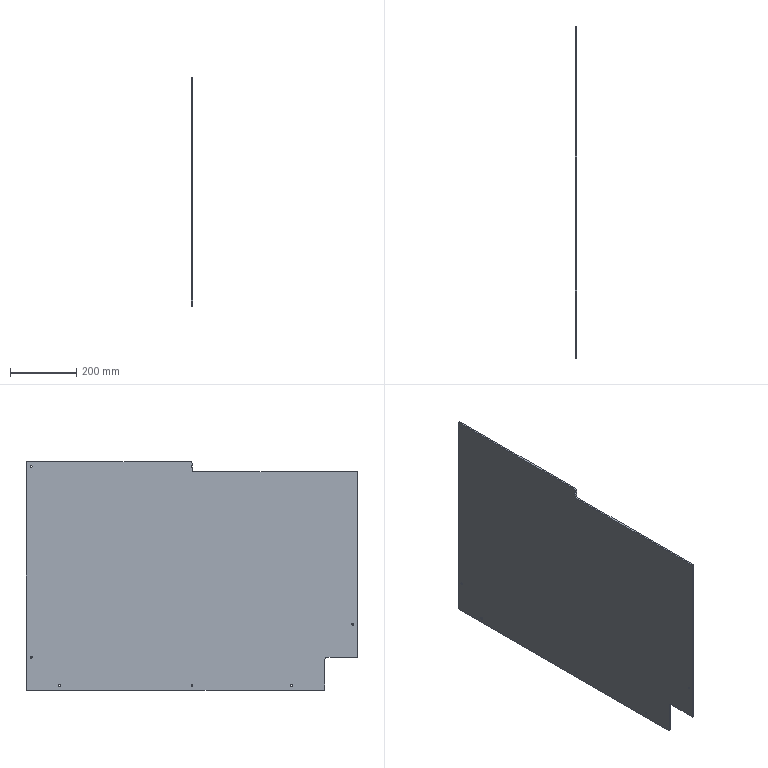Part | SolidWorks | features Chamfer 2, Fillet 2, ICE 2, Cut 1, Extrusion 1, HoleWzd 1 | 1 solid | 32 faces | box 5 x 1000 x 690 mm | volume 3324176 mm3 | cylinder 16 | plane 16 | commonest cylinder face diameters 6 x13 10 x2 20 x1
STEP:
#1=CARTESIAN_POINT('',(5.,485.,-248.));
#2=VERTEX_POINT('',#1);
#3=CARTESIAN_POINT('',(5.,485.,-242.));
#4=VERTEX_POINT('',#3);
#5=CARTESIAN_POINT('',(5.,485.,-245.));
#6=DIRECTION('',(-1.,0.,0.));
#7=DIRECTION('',(0.,0.,1.));
#8=AXIS2_PLACEMENT_3D('',#5,#6,#7);
#9=CIRCLE('',#8,3.);
#10=EDGE_CURVE('',#2,#4,#9,.T.);
#11=ORIENTED_EDGE('',*,*,#10,.F.);
#12=CARTESIAN_POINT('',(0.,485.,-248.));
#13=VERTEX_POINT('',#12);
#14=CARTESIAN_POINT('',(0.,485.,-248.));
#15=DIRECTION('',(-1.,0.,0.));
#16=VECTOR('',#15,1000.);
#17=LINE('',#14,#16);
#18=EDGE_CURVE('',#2,#13,#17,.T.);
#19=ORIENTED_EDGE('',*,*,#18,.T.);
#20=CARTESIAN_POINT('',(0.,485.,-242.));
#21=VERTEX_POINT('',#20);
#22=CARTESIAN_POINT('',(0.,485.,-245.));
#23=DIRECTION('',(-1.,0.,0.));
#24=DIRECTION('',(0.,0.,1.));
#25=AXIS2_PLACEMENT_3D('',#22,#23,#24);
#26=CIRCLE('',#25,3.);
#27=EDGE_CURVE('',#13,#21,#26,.T.);
#28=ORIENTED_EDGE('',*,*,#27,.T.);
#29=CARTESIAN_POINT('',(0.,485.,-242.));
#30=DIRECTION('',(-1.,0.,0.));
#31=VECTOR('',#30,1000.);
#32=LINE('',#29,#31);
#33=EDGE_CURVE('',#4,#21,#32,.T.);
#34=ORIENTED_EDGE('',*,*,#33,.F.);
#35=EDGE_LOOP('',(#11,#19,#28,#34));
#36=FACE_OUTER_BOUND('',#35,.T.);
#37=CARTESIAN_POINT('',(0.,485.,-245.));
#38=DIRECTION('',(-1.,0.,0.));
#39=DIRECTION('',(0.,0.,1.));
#40=AXIS2_PLACEMENT_3D('',#37,#38,#39);
#41=CYLINDRICAL_SURFACE('',#40,3.);
#42=ADVANCED_FACE('',(#36),#41,.F.);
#43=CARTESIAN_POINT('',(5.,400.,-333.));
#44=VERTEX_POINT('',#43);
#45=CARTESIAN_POINT('',(5.,400.,-327.));
#46=VERTEX_POINT('',#45);
#47=CARTESIAN_POINT('',(5.,400.,-330.));
#48=DIRECTION('',(-1.,0.,0.));
#49=DIRECTION('',(0.,0.,1.));
#50=AXIS2_PLACEMENT_3D('',#47,#48,#49);
#51=CIRCLE('',#50,3.);
#52=EDGE_CURVE('',#44,#46,#51,.T.);
#53=ORIENTED_EDGE('',*,*,#52,.F.);
#54=CARTESIAN_POINT('',(0.,400.,-333.));
#55=VERTEX_POINT('',#54);
#56=CARTESIAN_POINT('',(0.,400.,-333.));
#57=DIRECTION('',(-1.,0.,0.));
#58=VECTOR('',#57,1000.);
#59=LINE('',#56,#58);
#60=EDGE_CURVE('',#44,#55,#59,.T.);
#61=ORIENTED_EDGE('',*,*,#60,.T.);
#62=CARTESIAN_POINT('',(0.,400.,-327.));
#63=VERTEX_POINT('',#62);
#64=CARTESIAN_POINT('',(0.,400.,-330.));
#65=DIRECTION('',(-1.,0.,0.));
#66=DIRECTION('',(0.,0.,1.));
#67=AXIS2_PLACEMENT_3D('',#64,#65,#66);
#68=CIRCLE('',#67,3.);
#69=EDGE_CURVE('',#55,#63,#68,.T.);
#70=ORIENTED_EDGE('',*,*,#69,.T.);
#71=CARTESIAN_POINT('',(0.,400.,-327.));
#72=DIRECTION('',(-1.,0.,0.));
#73=VECTOR('',#72,1000.);
#74=LINE('',#71,#73);
#75=EDGE_CURVE('',#46,#63,#74,.T.);
#76=ORIENTED_EDGE('',*,*,#75,.F.);
#77=EDGE_LOOP('',(#53,#61,#70,#76));
#78=FACE_OUTER_BOUND('',#77,.T.);
#79=CARTESIAN_POINT('',(0.,400.,-330.));
#80=DIRECTION('',(-1.,0.,0.));
#81=DIRECTION('',(0.,0.,1.));
#82=AXIS2_PLACEMENT_3D('',#79,#80,#81);
#83=CYLINDRICAL_SURFACE('',#82,3.);
#84=ADVANCED_FACE('',(#78),#83,.F.);
#85=CARTESIAN_POINT('',(5.,-300.,-333.));
#86=VERTEX_POINT('',#85);
#87=CARTESIAN_POINT('',(5.,-300.,-327.));
#88=VERTEX_POINT('',#87);
#89=CARTESIAN_POINT('',(5.,-300.,-330.));
#90=DIRECTION('',(-1.,0.,0.));
#91=DIRECTION('',(0.,0.,1.));
#92=AXIS2_PLACEMENT_3D('',#89,#90,#91);
#93=CIRCLE('',#92,3.);
#94=EDGE_CURVE('',#86,#88,#93,.T.);
#95=ORIENTED_EDGE('',*,*,#94,.F.);
#96=CARTESIAN_POINT('',(0.,-300.,-333.));
#97=VERTEX_POINT('',#96);
#98=CARTESIAN_POINT('',(0.,-300.,-333.));
#99=DIRECTION('',(-1.,0.,0.));
#100=VECTOR('',#99,1000.);
#101=LINE('',#98,#100);
#102=EDGE_CURVE('',#86,#97,#101,.T.);
#103=ORIENTED_EDGE('',*,*,#102,.T.);
#104=CARTESIAN_POINT('',(0.,-300.,-327.));
#105=VERTEX_POINT('',#104);
#106=CARTESIAN_POINT('',(0.,-300.,-330.));
#107=DIRECTION('',(-1.,0.,0.));
#108=DIRECTION('',(0.,0.,1.));
#109=AXIS2_PLACEMENT_3D('',#106,#107,#108);
#110=CIRCLE('',#109,3.);
#111=EDGE_CURVE('',#97,#105,#110,.T.);
#112=ORIENTED_EDGE('',*,*,#111,.T.);
#113=CARTESIAN_POINT('',(0.,-300.,-327.));
#114=DIRECTION('',(-1.,0.,0.));
#115=VECTOR('',#114,1000.);
#116=LINE('',#113,#115);
#117=EDGE_CURVE('',#88,#105,#116,.T.);
#118=ORIENTED_EDGE('',*,*,#117,.F.);
#119=EDGE_LOOP('',(#95,#103,#112,#118));
#120=FACE_OUTER_BOUND('',#119,.T.);
#121=CARTESIAN_POINT('',(0.,-300.,-330.));
#122=DIRECTION('',(-1.,0.,0.));
#123=DIRECTION('',(0.,0.,1.));
#124=AXIS2_PLACEMENT_3D('',#121,#122,#123);
#125=CYLINDRICAL_SURFACE('',#124,3.);
#126=ADVANCED_FACE('',(#120),#125,.F.);
#127=CARTESIAN_POINT('',(5.,-485.,-148.));
#128=VERTEX_POINT('',#127);
#129=CARTESIAN_POINT('',(5.,-485.,-142.));
#130=VERTEX_POINT('',#129);
#131=CARTESIAN_POINT('',(5.,-485.,-145.));
#132=DIRECTION('',(-1.,0.,0.));
#133=DIRECTION('',(0.,0.,1.));
#134=AXIS2_PLACEMENT_3D('',#131,#132,#133);
#135=CIRCLE('',#134,3.);
#136=EDGE_CURVE('',#128,#130,#135,.T.);
#137=ORIENTED_EDGE('',*,*,#136,.F.);
#138=CARTESIAN_POINT('',(0.,-485.,-148.));
#139=VERTEX_POINT('',#138);
#140=CARTESIAN_POINT('',(0.,-485.,-148.));
#141=DIRECTION('',(-1.,0.,0.));
#142=VECTOR('',#141,1000.);
#143=LINE('',#140,#142);
#144=EDGE_CURVE('',#128,#139,#143,.T.);
#145=ORIENTED_EDGE('',*,*,#144,.T.);
#146=CARTESIAN_POINT('',(0.,-485.,-142.));
#147=VERTEX_POINT('',#146);
#148=CARTESIAN_POINT('',(0.,-485.,-145.));
#149=DIRECTION('',(-1.,0.,0.));
#150=DIRECTION('',(0.,0.,1.));
#151=AXIS2_PLACEMENT_3D('',#148,#149,#150);
#152=CIRCLE('',#151,3.);
#153=EDGE_CURVE('',#139,#147,#152,.T.);
#154=ORIENTED_EDGE('',*,*,#153,.T.);
#155=CARTESIAN_POINT('',(0.,-485.,-142.));
#156=DIRECTION('',(-1.,0.,0.));
#157=VECTOR('',#156,1000.);
#158=LINE('',#155,#157);
#159=EDGE_CURVE('',#130,#147,#158,.T.);
#160=ORIENTED_EDGE('',*,*,#159,.F.);
#161=EDGE_LOOP('',(#137,#145,#154,#160));
#162=FACE_OUTER_BOUND('',#161,.T.);
#163=CARTESIAN_POINT('',(0.,-485.,-145.));
#164=DIRECTION('',(-1.,0.,0.));
#165=DIRECTION('',(0.,0.,1.));
#166=AXIS2_PLACEMENT_3D('',#163,#164,#165);
#167=CYLINDRICAL_SURFACE('',#166,3.);
#168=ADVANCED_FACE('',(#162),#167,.F.);
#169=CARTESIAN_POINT('',(5.,0.,-333.));
#170=VERTEX_POINT('',#169);
#171=CARTESIAN_POINT('',(5.,0.,-327.));
#172=VERTEX_POINT('',#171);
#173=CARTESIAN_POINT('',(5.,0.,-330.));
#174=DIRECTION('',(-1.,0.,0.));
#175=DIRECTION('',(0.,0.,1.));
#176=AXIS2_PLACEMENT_3D('',#173,#174,#175);
#177=CIRCLE('',#176,3.);
#178=EDGE_CURVE('',#170,#172,#177,.T.);
#179=ORIENTED_EDGE('',*,*,#178,.F.);
#180=CARTESIAN_POINT('',(0.,0.,-333.));
#181=VERTEX_POINT('',#180);
#182=CARTESIAN_POINT('',(5.,0.,-333.));
#183=DIRECTION('',(-1.,0.,0.));
#184=VECTOR('',#183,1000.);
#185=LINE('',#182,#184);
#186=EDGE_CURVE('',#170,#181,#185,.T.);
#187=ORIENTED_EDGE('',*,*,#186,.T.);
#188=CARTESIAN_POINT('',(0.,0.,-327.));
#189=VERTEX_POINT('',#188);
#190=CARTESIAN_POINT('',(0.,0.,-330.));
#191=DIRECTION('',(-1.,0.,0.));
#192=DIRECTION('',(0.,0.,1.));
#193=AXIS2_PLACEMENT_3D('',#190,#191,#192);
#194=CIRCLE('',#193,3.);
#195=EDGE_CURVE('',#181,#189,#194,.T.);
#196=ORIENTED_EDGE('',*,*,#195,.T.);
#197=CARTESIAN_POINT('',(5.,0.,-327.));
#198=DIRECTION('',(-1.,0.,0.));
#199=VECTOR('',#198,1000.);
#200=LINE('',#197,#199);
#201=EDGE_CURVE('',#172,#189,#200,.T.);
#202=ORIENTED_EDGE('',*,*,#201,.F.);
#203=EDGE_LOOP('',(#179,#187,#196,#202));
#204=FACE_OUTER_BOUND('',#203,.T.);
#205=CARTESIAN_POINT('',(5.,0.,-330.));
#206=DIRECTION('',(-1.,0.,0.));
#207=DIRECTION('',(0.,0.,1.));
#208=AXIS2_PLACEMENT_3D('',#205,#206,#207);
#209=CYLINDRICAL_SURFACE('',#208,3.);
#210=ADVANCED_FACE('',(#204),#209,.F.);
#211=CARTESIAN_POINT('',(5.,485.,327.));
#212=VERTEX_POINT('',#211);
#213=CARTESIAN_POINT('',(5.,485.,333.));
#214=VERTEX_POINT('',#213);
#215=CARTESIAN_POINT('',(5.,485.,330.));
#216=DIRECTION('',(-1.,0.,0.));
#217=DIRECTION('',(0.,0.,-1.));
#218=AXIS2_PLACEMENT_3D('',#215,#216,#217);
#219=CIRCLE('',#218,3.);
#220=EDGE_CURVE('',#212,#214,#219,.T.);
#221=ORIENTED_EDGE('',*,*,#220,.F.);
#222=CARTESIAN_POINT('',(0.,485.,327.));
#223=VERTEX_POINT('',#222);
#224=CARTESIAN_POINT('',(5.,485.,327.));
#225=DIRECTION('',(-1.,0.,0.));
#226=VECTOR('',#225,1000.);
#227=LINE('',#224,#226);
#228=EDGE_CURVE('',#212,#223,#227,.T.);
#229=ORIENTED_EDGE('',*,*,#228,.T.);
#230=CARTESIAN_POINT('',(0.,485.,333.));
#231=VERTEX_POINT('',#230);
#232=CARTESIAN_POINT('',(0.,485.,330.));
#233=DIRECTION('',(-1.,0.,0.));
#234=DIRECTION('',(0.,0.,-1.));
#235=AXIS2_PLACEMENT_3D('',#232,#233,#234);
#236=CIRCLE('',#235,3.);
#237=EDGE_CURVE('',#223,#231,#236,.T.);
#238=ORIENTED_EDGE('',*,*,#237,.T.);
#239=CARTESIAN_POINT('',(5.,485.,333.));
#240=DIRECTION('',(-1.,0.,0.));
#241=VECTOR('',#240,1000.);
#242=LINE('',#239,#241);
#243=EDGE_CURVE('',#214,#231,#242,.T.);
#244=ORIENTED_EDGE('',*,*,#243,.F.);
#245=EDGE_LOOP('',(#221,#229,#238,#244));
#246=FACE_OUTER_BOUND('',#245,.T.);
#247=CARTESIAN_POINT('',(5.,485.,330.));
#248=DIRECTION('',(-1.,0.,0.));
#249=DIRECTION('',(0.,0.,1.));
#250=AXIS2_PLACEMENT_3D('',#247,#248,#249);
#251=CYLINDRICAL_SURFACE('',#250,3.);
#252=ADVANCED_FACE('',(#246),#251,.F.);
#253=CARTESIAN_POINT('',(0.,499.,345.));
#254=VERTEX_POINT('',#253);
#255=CARTESIAN_POINT('',(0.,5.,345.));
#256=VERTEX_POINT('',#255);
#257=CARTESIAN_POINT('',(0.,500.,345.));
#258=DIRECTION('',(0.,-1.,0.));
#259=VECTOR('',#258,1000.);
#260=LINE('',#257,#259);
#261=EDGE_CURVE('',#254,#256,#260,.T.);
#262=ORIENTED_EDGE('',*,*,#261,.T.);
#263=CARTESIAN_POINT('',(5.,5.,345.));
#264=VERTEX_POINT('',#263);
#265=CARTESIAN_POINT('',(5.,5.,345.));
#266=DIRECTION('',(1.,0.,0.));
#267=VECTOR('',#266,1000.);
#268=LINE('',#265,#267);
#269=EDGE_CURVE('',#256,#264,#268,.T.);
#270=ORIENTED_EDGE('',*,*,#269,.T.);
#271=CARTESIAN_POINT('',(5.,499.,345.));
#272=VERTEX_POINT('',#271);
#273=CARTESIAN_POINT('',(5.,500.,345.));
#274=DIRECTION('',(0.,-1.,0.));
#275=VECTOR('',#274,1000.);
#276=LINE('',#273,#275);
#277=EDGE_CURVE('',#272,#264,#276,.T.);
#278=ORIENTED_EDGE('',*,*,#277,.F.);
#279=CARTESIAN_POINT('',(5.,499.,345.));
#280=DIRECTION('',(-1.,0.,0.));
#281=VECTOR('',#280,1000.);
#282=LINE('',#279,#281);
#283=EDGE_CURVE('',#272,#254,#282,.T.);
#284=ORIENTED_EDGE('',*,*,#283,.T.);
#285=EDGE_LOOP('',(#262,#270,#278,#284));
#286=FACE_OUTER_BOUND('',#285,.T.);
#287=CARTESIAN_POINT('',(5.,500.,345.));
#288=DIRECTION('',(0.,0.,-1.));
#289=DIRECTION('',(0.,1.,0.));
#290=AXIS2_PLACEMENT_3D('',#287,#288,#289);
#291=PLANE('',#290);
#292=ADVANCED_FACE('',(#286),#291,.F.);
#293=CARTESIAN_POINT('',(0.,-500.,314.));
#294=VERTEX_POINT('',#293);
#295=CARTESIAN_POINT('',(0.,-500.,-244.));
#296=VERTEX_POINT('',#295);
#297=CARTESIAN_POINT('',(0.,-500.,-345.));
#298=DIRECTION('',(0.,0.,-1.));
#299=VECTOR('',#298,1000.);
#300=LINE('',#297,#299);
#301=EDGE_CURVE('',#294,#296,#300,.T.);
#302=ORIENTED_EDGE('',*,*,#301,.T.);
#303=CARTESIAN_POINT('',(5.,-500.,-244.));
#304=VERTEX_POINT('',#303);
#305=CARTESIAN_POINT('',(5.,-500.,-244.));
#306=DIRECTION('',(1.,0.,0.));
#307=VECTOR('',#306,1000.);
#308=LINE('',#305,#307);
#309=EDGE_CURVE('',#296,#304,#308,.T.);
#310=ORIENTED_EDGE('',*,*,#309,.T.);
#311=CARTESIAN_POINT('',(5.,-500.,314.));
#312=VERTEX_POINT('',#311);
#313=CARTESIAN_POINT('',(5.,-500.,-345.));
#314=DIRECTION('',(0.,0.,-1.));
#315=VECTOR('',#314,1000.);
#316=LINE('',#313,#315);
#317=EDGE_CURVE('',#312,#304,#316,.T.);
#318=ORIENTED_EDGE('',*,*,#317,.F.);
#319=CARTESIAN_POINT('',(5.,-500.,314.));
#320=DIRECTION('',(-1.,0.,0.));
#321=VECTOR('',#320,1000.);
#322=LINE('',#319,#321);
#323=EDGE_CURVE('',#312,#294,#322,.T.);
#324=ORIENTED_EDGE('',*,*,#323,.T.);
#325=EDGE_LOOP('',(#302,#310,#318,#324));
#326=FACE_OUTER_BOUND('',#325,.T.);
#327=CARTESIAN_POINT('',(5.,-500.,-345.));
#328=DIRECTION('',(0.,1.,0.));
#329=DIRECTION('',(0.,0.,1.));
#330=AXIS2_PLACEMENT_3D('',#327,#328,#329);
#331=PLANE('',#330);
#332=ADVANCED_FACE('',(#326),#331,.F.);
#333=CARTESIAN_POINT('',(5.,-399.,-345.));
#334=VERTEX_POINT('',#333);
#335=CARTESIAN_POINT('',(5.,499.,-345.));
#336=VERTEX_POINT('',#335);
#337=CARTESIAN_POINT('',(5.,500.,-345.));
#338=DIRECTION('',(0.,1.,0.));
#339=VECTOR('',#338,1000.);
#340=LINE('',#337,#339);
#341=EDGE_CURVE('',#334,#336,#340,.T.);
#342=ORIENTED_EDGE('',*,*,#341,.F.);
#343=CARTESIAN_POINT('',(0.,-399.,-345.));
#344=VERTEX_POINT('',#343);
#345=CARTESIAN_POINT('',(5.,-399.,-345.));
#346=DIRECTION('',(-1.,0.,0.));
#347=VECTOR('',#346,1000.);
#348=LINE('',#345,#347);
#349=EDGE_CURVE('',#334,#344,#348,.T.);
#350=ORIENTED_EDGE('',*,*,#349,.T.);
#351=CARTESIAN_POINT('',(0.,499.,-345.));
#352=VERTEX_POINT('',#351);
#353=CARTESIAN_POINT('',(0.,500.,-345.));
#354=DIRECTION('',(0.,1.,0.));
#355=VECTOR('',#354,1000.);
#356=LINE('',#353,#355);
#357=EDGE_CURVE('',#344,#352,#356,.T.);
#358=ORIENTED_EDGE('',*,*,#357,.T.);
#359=CARTESIAN_POINT('',(5.,499.,-345.));
#360=DIRECTION('',(1.,0.,0.));
#361=VECTOR('',#360,1000.);
#362=LINE('',#359,#361);
#363=EDGE_CURVE('',#352,#336,#362,.T.);
#364=ORIENTED_EDGE('',*,*,#363,.T.);
#365=EDGE_LOOP('',(#342,#350,#358,#364));
#366=FACE_OUTER_BOUND('',#365,.T.);
#367=CARTESIAN_POINT('',(5.,500.,-345.));
#368=DIRECTION('',(0.,0.,1.));
#369=DIRECTION('',(0.,-1.,0.));
#370=AXIS2_PLACEMENT_3D('',#367,#368,#369);
#371=PLANE('',#370);
#372=ADVANCED_FACE('',(#366),#371,.F.);
#373=CARTESIAN_POINT('',(5.,500.,-344.));
#374=VERTEX_POINT('',#373);
#375=CARTESIAN_POINT('',(5.,500.,344.));
#376=VERTEX_POINT('',#375);
#377=CARTESIAN_POINT('',(5.,500.,-345.));
#378=DIRECTION('',(0.,0.,1.));
#379=VECTOR('',#378,1000.);
#380=LINE('',#377,#379);
#381=EDGE_CURVE('',#374,#376,#380,.T.);
#382=ORIENTED_EDGE('',*,*,#381,.F.);
#383=CARTESIAN_POINT('',(0.,500.,-344.));
#384=VERTEX_POINT('',#383);
#385=CARTESIAN_POINT('',(5.,500.,-344.));
#386=DIRECTION('',(-1.,0.,0.));
#387=VECTOR('',#386,1000.);
#388=LINE('',#385,#387);
#389=EDGE_CURVE('',#374,#384,#388,.T.);
#390=ORIENTED_EDGE('',*,*,#389,.T.);
#391=CARTESIAN_POINT('',(0.,500.,344.));
#392=VERTEX_POINT('',#391);
#393=CARTESIAN_POINT('',(0.,500.,-345.));
#394=DIRECTION('',(0.,0.,1.));
#395=VECTOR('',#394,1000.);
#396=LINE('',#393,#395);
#397=EDGE_CURVE('',#384,#392,#396,.T.);
#398=ORIENTED_EDGE('',*,*,#397,.T.);
#399=CARTESIAN_POINT('',(5.,500.,344.));
#400=DIRECTION('',(1.,0.,0.));
#401=VECTOR('',#400,1000.);
#402=LINE('',#399,#401);
#403=EDGE_CURVE('',#392,#376,#402,.T.);
#404=ORIENTED_EDGE('',*,*,#403,.T.);
#405=EDGE_LOOP('',(#382,#390,#398,#404));
#406=FACE_OUTER_BOUND('',#405,.T.);
#407=CARTESIAN_POINT('',(5.,500.,-345.));
#408=DIRECTION('',(0.,-1.,0.));
#409=DIRECTION('',(0.,0.,-1.));
#410=AXIS2_PLACEMENT_3D('',#407,#408,#409);
#411=PLANE('',#410);
#412=ADVANCED_FACE('',(#406),#411,.F.);
#413=CARTESIAN_POINT('',(5.,485.,-245.));
#414=DIRECTION('',(-1.,0.,0.));
#415=DIRECTION('',(0.,0.,1.));
#416=AXIS2_PLACEMENT_3D('',#413,#414,#415);
#417=CIRCLE('',#416,3.);
#418=EDGE_CURVE('',#4,#2,#417,.T.);
#419=ORIENTED_EDGE('',*,*,#418,.T.);
#420=ORIENTED_EDGE('',*,*,#10,.T.);
#421=EDGE_LOOP('',(#419,#420));
#422=FACE_BOUND('',#421,.T.);
#423=CARTESIAN_POINT('',(5.,400.,-330.));
#424=DIRECTION('',(-1.,0.,0.));
#425=DIRECTION('',(0.,0.,1.));
#426=AXIS2_PLACEMENT_3D('',#423,#424,#425);
#427=CIRCLE('',#426,3.);
#428=EDGE_CURVE('',#46,#44,#427,.T.);
#429=ORIENTED_EDGE('',*,*,#428,.T.);
#430=ORIENTED_EDGE('',*,*,#52,.T.);
#431=EDGE_LOOP('',(#429,#430));
#432=FACE_BOUND('',#431,.T.);
#433=CARTESIAN_POINT('',(5.,-300.,-330.));
#434=DIRECTION('',(-1.,0.,0.));
#435=DIRECTION('',(0.,0.,1.));
#436=AXIS2_PLACEMENT_3D('',#433,#434,#435);
#437=CIRCLE('',#436,3.);
#438=EDGE_CURVE('',#88,#86,#437,.T.);
#439=ORIENTED_EDGE('',*,*,#438,.T.);
#440=ORIENTED_EDGE('',*,*,#94,.T.);
#441=EDGE_LOOP('',(#439,#440));
#442=FACE_BOUND('',#441,.T.);
#443=CARTESIAN_POINT('',(5.,-485.,-145.));
#444=DIRECTION('',(-1.,0.,0.));
#445=DIRECTION('',(0.,0.,1.));
#446=AXIS2_PLACEMENT_3D('',#443,#444,#445);
#447=CIRCLE('',#446,3.);
#448=EDGE_CURVE('',#130,#128,#447,.T.);
#449=ORIENTED_EDGE('',*,*,#448,.T.);
#450=ORIENTED_EDGE('',*,*,#136,.T.);
#451=EDGE_LOOP('',(#449,#450));
#452=FACE_BOUND('',#451,.T.);
#453=CARTESIAN_POINT('',(5.,0.,-330.));
#454=DIRECTION('',(-1.,0.,0.));
#455=DIRECTION('',(0.,0.,1.));
#456=AXIS2_PLACEMENT_3D('',#453,#454,#455);
#457=CIRCLE('',#456,3.);
#458=EDGE_CURVE('',#172,#170,#457,.T.);
#459=ORIENTED_EDGE('',*,*,#458,.T.);
#460=ORIENTED_EDGE('',*,*,#178,.T.);
#461=EDGE_LOOP('',(#459,#460));
#462=FACE_BOUND('',#461,.T.);
#463=ORIENTED_EDGE('',*,*,#277,.T.);
#464=CARTESIAN_POINT('',(5.,0.,340.));
#465=VERTEX_POINT('',#464);
#466=CARTESIAN_POINT('',(5.,5.,340.));
#467=DIRECTION('',(1.,0.,0.));
#468=DIRECTION('',(0.,0.,1.));
#469=AXIS2_PLACEMENT_3D('',#466,#467,#468);
#470=CIRCLE('',#469,5.);
#471=EDGE_CURVE('',#264,#465,#470,.T.);
#472=ORIENTED_EDGE('',*,*,#471,.T.);
#473=CARTESIAN_POINT('',(5.,0.,333.));
#474=VERTEX_POINT('',#473);
#475=CARTESIAN_POINT('',(5.,0.,345.));
#476=DIRECTION('',(0.,0.,-1.));
#477=VECTOR('',#476,1000.);
#478=LINE('',#475,#477);
#479=EDGE_CURVE('',#465,#474,#478,.T.);
#480=ORIENTED_EDGE('',*,*,#479,.T.);
#481=CARTESIAN_POINT('',(5.,0.,327.));
#482=VERTEX_POINT('',#481);
#483=CARTESIAN_POINT('',(5.,0.,330.));
#484=DIRECTION('',(-1.,0.,0.));
#485=DIRECTION('',(0.,0.,1.));
#486=AXIS2_PLACEMENT_3D('',#483,#484,#485);
#487=CIRCLE('',#486,3.);
#488=EDGE_CURVE('',#474,#482,#487,.T.);
#489=ORIENTED_EDGE('',*,*,#488,.T.);
#490=CARTESIAN_POINT('',(5.,0.,320.));
#491=VERTEX_POINT('',#490);
#492=CARTESIAN_POINT('',(5.,0.,345.));
#493=DIRECTION('',(0.,0.,-1.));
#494=VECTOR('',#493,1000.);
#495=LINE('',#492,#494);
#496=EDGE_CURVE('',#482,#491,#495,.T.);
#497=ORIENTED_EDGE('',*,*,#496,.T.);
#498=CARTESIAN_POINT('',(5.,-5.,315.));
#499=VERTEX_POINT('',#498);
#500=CARTESIAN_POINT('',(5.,-5.,320.));
#501=DIRECTION('',(-1.,0.,0.));
#502=DIRECTION('',(0.,0.,1.));
#503=AXIS2_PLACEMENT_3D('',#500,#501,#502);
#504=CIRCLE('',#503,5.);
#505=EDGE_CURVE('',#491,#499,#504,.T.);
#506=ORIENTED_EDGE('',*,*,#505,.T.);
#507=CARTESIAN_POINT('',(5.,-499.,315.));
#508=VERTEX_POINT('',#507);
#509=CARTESIAN_POINT('',(5.,-500.,315.));
#510=DIRECTION('',(0.,-1.,0.));
#511=VECTOR('',#510,1000.);
#512=LINE('',#509,#511);
#513=EDGE_CURVE('',#499,#508,#512,.T.);
#514=ORIENTED_EDGE('',*,*,#513,.T.);
#515=CARTESIAN_POINT('',(5.,-500.,314.));
#516=DIRECTION('',(0.,-0.7071,-0.7071));
#517=VECTOR('',#516,1000.);
#518=LINE('',#515,#517);
#519=EDGE_CURVE('',#508,#312,#518,.T.);
#520=ORIENTED_EDGE('',*,*,#519,.T.);
#521=ORIENTED_EDGE('',*,*,#317,.T.);
#522=CARTESIAN_POINT('',(5.,-499.,-245.));
#523=VERTEX_POINT('',#522);
#524=CARTESIAN_POINT('',(5.,-499.,-245.));
#525=DIRECTION('',(0.,0.7071,-0.7071));
#526=VECTOR('',#525,1000.);
#527=LINE('',#524,#526);
#528=EDGE_CURVE('',#304,#523,#527,.T.);
#529=ORIENTED_EDGE('',*,*,#528,.T.);
#530=CARTESIAN_POINT('',(5.,-410.,-245.));
#531=VERTEX_POINT('',#530);
#532=CARTESIAN_POINT('',(5.,-500.,-245.));
#533=DIRECTION('',(0.,1.,0.));
#534=VECTOR('',#533,1000.);
#535=LINE('',#532,#534);
#536=EDGE_CURVE('',#523,#531,#535,.T.);
#537=ORIENTED_EDGE('',*,*,#536,.T.);
#538=CARTESIAN_POINT('',(5.,-400.,-255.));
#539=VERTEX_POINT('',#538);
#540=CARTESIAN_POINT('',(5.,-410.,-255.));
#541=DIRECTION('',(-1.,0.,0.));
#542=DIRECTION('',(0.,0.,1.));
#543=AXIS2_PLACEMENT_3D('',#540,#541,#542);
#544=CIRCLE('',#543,10.);
#545=EDGE_CURVE('',#531,#539,#544,.T.);
#546=ORIENTED_EDGE('',*,*,#545,.T.);
#547=CARTESIAN_POINT('',(5.,-400.,-344.));
#548=VERTEX_POINT('',#547);
#549=CARTESIAN_POINT('',(5.,-400.,-245.));
#550=DIRECTION('',(0.,0.,-1.));
#551=VECTOR('',#550,1000.);
#552=LINE('',#549,#551);
#553=EDGE_CURVE('',#539,#548,#552,.T.);
#554=ORIENTED_EDGE('',*,*,#553,.T.);
#555=CARTESIAN_POINT('',(5.,-399.,-345.));
#556=DIRECTION('',(0.,0.7071,-0.7071));
#557=VECTOR('',#556,1000.);
#558=LINE('',#555,#557);
#559=EDGE_CURVE('',#548,#334,#558,.T.);
#560=ORIENTED_EDGE('',*,*,#559,.T.);
#561=ORIENTED_EDGE('',*,*,#341,.T.);
#562=CARTESIAN_POINT('',(5.,500.,-344.));
#563=DIRECTION('',(0.,0.7071,0.7071));
#564=VECTOR('',#563,1000.);
#565=LINE('',#562,#564);
#566=EDGE_CURVE('',#336,#374,#565,.T.);
#567=ORIENTED_EDGE('',*,*,#566,.T.);
#568=ORIENTED_EDGE('',*,*,#381,.T.);
#569=CARTESIAN_POINT('',(5.,499.,345.));
#570=DIRECTION('',(0.,-0.7071,0.7071));
#571=VECTOR('',#570,1000.);
#572=LINE('',#569,#571);
#573=EDGE_CURVE('',#376,#272,#572,.T.);
#574=ORIENTED_EDGE('',*,*,#573,.T.);
#575=EDGE_LOOP('',(#463,#472,#480,#489,#497,#506,#514,#520,#521,#529,#537,#546,#554,#560,#561,#567,#568,#574));
#576=FACE_OUTER_BOUND('',#575,.T.);
#577=CARTESIAN_POINT('',(5.,485.,330.));
#578=DIRECTION('',(-1.,0.,0.));
#579=DIRECTION('',(0.,0.,-1.));
#580=AXIS2_PLACEMENT_3D('',#577,#578,#579);
#581=CIRCLE('',#580,3.);
#582=EDGE_CURVE('',#214,#212,#581,.T.);
#583=ORIENTED_EDGE('',*,*,#582,.T.);
#584=ORIENTED_EDGE('',*,*,#220,.T.);
#585=EDGE_LOOP('',(#583,#584));
#586=FACE_BOUND('',#585,.T.);
#587=CARTESIAN_POINT('',(5.,-500.,345.));
#588=DIRECTION('',(-1.,0.,0.));
#589=DIRECTION('',(0.,0.,1.));
#590=AXIS2_PLACEMENT_3D('',#587,#588,#589);
#591=PLANE('',#590);
#592=ADVANCED_FACE('',(#422,#432,#442,#452,#462,#576,#586),#591,.F.);
#593=CARTESIAN_POINT('',(0.,0.,340.));
#594=VERTEX_POINT('',#593);
#595=CARTESIAN_POINT('',(0.,0.,333.));
#596=VERTEX_POINT('',#595);
#597=CARTESIAN_POINT('',(0.,0.,345.));
#598=DIRECTION('',(0.,0.,-1.));
#599=VECTOR('',#598,1000.);
#600=LINE('',#597,#599);
#601=EDGE_CURVE('',#594,#596,#600,.T.);
#602=ORIENTED_EDGE('',*,*,#601,.F.);
#603=CARTESIAN_POINT('',(0.,5.,340.));
#604=DIRECTION('',(-1.,0.,0.));
#605=DIRECTION('',(0.,0.,1.));
#606=AXIS2_PLACEMENT_3D('',#603,#604,#605);
#607=CIRCLE('',#606,5.);
#608=EDGE_CURVE('',#594,#256,#607,.T.);
#609=ORIENTED_EDGE('',*,*,#608,.T.);
#610=ORIENTED_EDGE('',*,*,#261,.F.);
#611=CARTESIAN_POINT('',(0.,-0.5,844.5));
#612=DIRECTION('',(0.,0.7071,-0.7071));
#613=VECTOR('',#612,1000.);
#614=LINE('',#611,#613);
#615=EDGE_CURVE('',#254,#392,#614,.T.);
#616=ORIENTED_EDGE('',*,*,#615,.T.);
#617=ORIENTED_EDGE('',*,*,#397,.F.);
#618=CARTESIAN_POINT('',(0.,344.5,-499.5));
#619=DIRECTION('',(0.,-0.7071,-0.7071));
#620=VECTOR('',#619,1000.);
#621=LINE('',#618,#620);
#622=EDGE_CURVE('',#384,#352,#621,.T.);
#623=ORIENTED_EDGE('',*,*,#622,.T.);
#624=ORIENTED_EDGE('',*,*,#357,.F.);
#625=CARTESIAN_POINT('',(0.,-400.,-344.));
#626=VERTEX_POINT('',#625);
#627=CARTESIAN_POINT('',(0.,-794.5,50.5));
#628=DIRECTION('',(0.,-0.7071,0.7071));
#629=VECTOR('',#628,1000.);
#630=LINE('',#627,#629);
#631=EDGE_CURVE('',#344,#626,#630,.T.);
#632=ORIENTED_EDGE('',*,*,#631,.T.);
#633=CARTESIAN_POINT('',(0.,-400.,-255.));
#634=VERTEX_POINT('',#633);
#635=CARTESIAN_POINT('',(0.,-400.,-245.));
#636=DIRECTION('',(0.,0.,-1.));
#637=VECTOR('',#636,1000.);
#638=LINE('',#635,#637);
#639=EDGE_CURVE('',#634,#626,#638,.T.);
#640=ORIENTED_EDGE('',*,*,#639,.F.);
#641=CARTESIAN_POINT('',(0.,-410.,-245.));
#642=VERTEX_POINT('',#641);
#643=CARTESIAN_POINT('',(0.,-410.,-255.));
#644=DIRECTION('',(1.,0.,0.));
#645=DIRECTION('',(0.,0.,1.));
#646=AXIS2_PLACEMENT_3D('',#643,#644,#645);
#647=CIRCLE('',#646,10.);
#648=EDGE_CURVE('',#634,#642,#647,.T.);
#649=ORIENTED_EDGE('',*,*,#648,.T.);
#650=CARTESIAN_POINT('',(0.,-499.,-245.));
#651=VERTEX_POINT('',#650);
#652=CARTESIAN_POINT('',(0.,-500.,-245.));
#653=DIRECTION('',(0.,1.,0.));
#654=VECTOR('',#653,1000.);
#655=LINE('',#652,#654);
#656=EDGE_CURVE('',#651,#642,#655,.T.);
#657=ORIENTED_EDGE('',*,*,#656,.F.);
#658=CARTESIAN_POINT('',(0.,-794.5,50.5));
#659=DIRECTION('',(0.,-0.7071,0.7071));
#660=VECTOR('',#659,1000.);
#661=LINE('',#658,#660);
#662=EDGE_CURVE('',#651,#296,#661,.T.);
#663=ORIENTED_EDGE('',*,*,#662,.T.);
#664=ORIENTED_EDGE('',*,*,#301,.F.);
#665=CARTESIAN_POINT('',(0.,-499.,315.));
#666=VERTEX_POINT('',#665);
#667=CARTESIAN_POINT('',(0.,-484.5,329.5));
#668=DIRECTION('',(0.,0.7071,0.7071));
#669=VECTOR('',#668,1000.);
#670=LINE('',#667,#669);
#671=EDGE_CURVE('',#294,#666,#670,.T.);
#672=ORIENTED_EDGE('',*,*,#671,.T.);
#673=CARTESIAN_POINT('',(0.,-5.,315.));
#674=VERTEX_POINT('',#673);
#675=CARTESIAN_POINT('',(0.,-500.,315.));
#676=DIRECTION('',(0.,-1.,0.));
#677=VECTOR('',#676,1000.);
#678=LINE('',#675,#677);
#679=EDGE_CURVE('',#674,#666,#678,.T.);
#680=ORIENTED_EDGE('',*,*,#679,.F.);
#681=CARTESIAN_POINT('',(0.,0.,320.));
#682=VERTEX_POINT('',#681);
#683=CARTESIAN_POINT('',(0.,-5.,320.));
#684=DIRECTION('',(1.,0.,0.));
#685=DIRECTION('',(0.,0.,1.));
#686=AXIS2_PLACEMENT_3D('',#683,#684,#685);
#687=CIRCLE('',#686,5.);
#688=EDGE_CURVE('',#674,#682,#687,.T.);
#689=ORIENTED_EDGE('',*,*,#688,.T.);
#690=CARTESIAN_POINT('',(0.,0.,327.));
#691=VERTEX_POINT('',#690);
#692=CARTESIAN_POINT('',(0.,0.,345.));
#693=DIRECTION('',(0.,0.,-1.));
#694=VECTOR('',#693,1000.);
#695=LINE('',#692,#694);
#696=EDGE_CURVE('',#691,#682,#695,.T.);
#697=ORIENTED_EDGE('',*,*,#696,.F.);
#698=CARTESIAN_POINT('',(0.,0.,330.));
#699=DIRECTION('',(-1.,0.,0.));
#700=DIRECTION('',(0.,0.,1.));
#701=AXIS2_PLACEMENT_3D('',#698,#699,#700);
#702=CIRCLE('',#701,3.);
#703=EDGE_CURVE('',#596,#691,#702,.T.);
#704=ORIENTED_EDGE('',*,*,#703,.F.);
#705=EDGE_LOOP('',(#602,#609,#610,#616,#617,#623,#624,#632,#640,#649,#657,#663,#664,#672,#680,#689,#697,#704));
#706=FACE_OUTER_BOUND('',#705,.T.);
#707=CARTESIAN_POINT('',(0.,485.,-245.));
#708=DIRECTION('',(-1.,0.,0.));
#709=DIRECTION('',(0.,0.,1.));
#710=AXIS2_PLACEMENT_3D('',#707,#708,#709);
#711=CIRCLE('',#710,3.);
#712=EDGE_CURVE('',#21,#13,#711,.T.);
#713=ORIENTED_EDGE('',*,*,#712,.F.);
#714=ORIENTED_EDGE('',*,*,#27,.F.);
#715=EDGE_LOOP('',(#713,#714));
#716=FACE_BOUND('',#715,.T.);
#717=CARTESIAN_POINT('',(0.,400.,-330.));
#718=DIRECTION('',(-1.,0.,0.));
#719=DIRECTION('',(0.,0.,1.));
#720=AXIS2_PLACEMENT_3D('',#717,#718,#719);
#721=CIRCLE('',#720,3.);
#722=EDGE_CURVE('',#63,#55,#721,.T.);
#723=ORIENTED_EDGE('',*,*,#722,.F.);
#724=ORIENTED_EDGE('',*,*,#69,.F.);
#725=EDGE_LOOP('',(#723,#724));
#726=FACE_BOUND('',#725,.T.);
#727=CARTESIAN_POINT('',(0.,-300.,-330.));
#728=DIRECTION('',(-1.,0.,0.));
#729=DIRECTION('',(0.,0.,1.));
#730=AXIS2_PLACEMENT_3D('',#727,#728,#729);
#731=CIRCLE('',#730,3.);
#732=EDGE_CURVE('',#105,#97,#731,.T.);
#733=ORIENTED_EDGE('',*,*,#732,.F.);
#734=ORIENTED_EDGE('',*,*,#111,.F.);
#735=EDGE_LOOP('',(#733,#734));
#736=FACE_BOUND('',#735,.T.);
#737=CARTESIAN_POINT('',(0.,-485.,-145.));
#738=DIRECTION('',(-1.,0.,0.));
#739=DIRECTION('',(0.,0.,1.));
#740=AXIS2_PLACEMENT_3D('',#737,#738,#739);
#741=CIRCLE('',#740,3.);
#742=EDGE_CURVE('',#147,#139,#741,.T.);
#743=ORIENTED_EDGE('',*,*,#742,.F.);
#744=ORIENTED_EDGE('',*,*,#153,.F.);
#745=EDGE_LOOP('',(#743,#744));
#746=FACE_BOUND('',#745,.T.);
#747=CARTESIAN_POINT('',(0.,0.,-330.));
#748=DIRECTION('',(-1.,0.,0.));
#749=DIRECTION('',(0.,0.,1.));
#750=AXIS2_PLACEMENT_3D('',#747,#748,#749);
#751=CIRCLE('',#750,3.);
#752=EDGE_CURVE('',#189,#181,#751,.T.);
#753=ORIENTED_EDGE('',*,*,#752,.F.);
#754=ORIENTED_EDGE('',*,*,#195,.F.);
#755=EDGE_LOOP('',(#753,#754));
#756=FACE_BOUND('',#755,.T.);
#757=CARTESIAN_POINT('',(0.,485.,330.));
#758=DIRECTION('',(-1.,0.,0.));
#759=DIRECTION('',(0.,0.,-1.));
#760=AXIS2_PLACEMENT_3D('',#757,#758,#759);
#761=CIRCLE('',#760,3.);
#762=EDGE_CURVE('',#231,#223,#761,.T.);
#763=ORIENTED_EDGE('',*,*,#762,.F.);
#764=ORIENTED_EDGE('',*,*,#237,.F.);
#765=EDGE_LOOP('',(#763,#764));
#766=FACE_BOUND('',#765,.T.);
#767=CARTESIAN_POINT('',(0.,-500.,345.));
#768=DIRECTION('',(-1.,0.,0.));
#769=DIRECTION('',(0.,0.,1.));
#770=AXIS2_PLACEMENT_3D('',#767,#768,#769);
#771=PLANE('',#770);
#772=ADVANCED_FACE('',(#706,#716,#726,#736,#746,#756,#766),#771,.T.);
#773=ORIENTED_EDGE('',*,*,#566,.F.);
#774=ORIENTED_EDGE('',*,*,#363,.F.);
#775=ORIENTED_EDGE('',*,*,#622,.F.);
#776=ORIENTED_EDGE('',*,*,#389,.F.);
#777=EDGE_LOOP('',(#773,#774,#775,#776));
#778=FACE_OUTER_BOUND('',#777,.T.);
#779=CARTESIAN_POINT('',(5.,500.,-344.));
#780=DIRECTION('',(0.,-0.7071,0.7071));
#781=DIRECTION('',(0.,-0.7071,-0.7071));
#782=AXIS2_PLACEMENT_3D('',#779,#780,#781);
#783=PLANE('',#782);
#784=ADVANCED_FACE('',(#778),#783,.F.);
#785=ORIENTED_EDGE('',*,*,#573,.F.);
#786=ORIENTED_EDGE('',*,*,#403,.F.);
#787=ORIENTED_EDGE('',*,*,#615,.F.);
#788=ORIENTED_EDGE('',*,*,#283,.F.);
#789=EDGE_LOOP('',(#785,#786,#787,#788));
#790=FACE_OUTER_BOUND('',#789,.T.);
#791=CARTESIAN_POINT('',(5.,499.,345.));
#792=DIRECTION('',(0.,-0.7071,-0.7071));
#793=DIRECTION('',(0.,0.7071,-0.7071));
#794=AXIS2_PLACEMENT_3D('',#791,#792,#793);
#795=PLANE('',#794);
#796=ADVANCED_FACE('',(#790),#795,.F.);
#797=ORIENTED_EDGE('',*,*,#228,.F.);
#798=ORIENTED_EDGE('',*,*,#582,.F.);
#799=ORIENTED_EDGE('',*,*,#243,.T.);
#800=ORIENTED_EDGE('',*,*,#762,.T.);
#801=EDGE_LOOP('',(#797,#798,#799,#800));
#802=FACE_OUTER_BOUND('',#801,.T.);
#803=CARTESIAN_POINT('',(5.,485.,330.));
#804=DIRECTION('',(-1.,0.,0.));
#805=DIRECTION('',(0.,0.,1.));
#806=AXIS2_PLACEMENT_3D('',#803,#804,#805);
#807=CYLINDRICAL_SURFACE('',#806,3.);
#808=ADVANCED_FACE('',(#802),#807,.F.);
#809=ORIENTED_EDGE('',*,*,#703,.T.);
#810=CARTESIAN_POINT('',(5.,0.,327.));
#811=DIRECTION('',(1.,0.,0.));
#812=VECTOR('',#811,1000.);
#813=LINE('',#810,#812);
#814=EDGE_CURVE('',#691,#482,#813,.T.);
#815=ORIENTED_EDGE('',*,*,#814,.T.);
#816=ORIENTED_EDGE('',*,*,#488,.F.);
#817=CARTESIAN_POINT('',(5.,0.,333.));
#818=DIRECTION('',(-1.,0.,0.));
#819=VECTOR('',#818,1000.);
#820=LINE('',#817,#819);
#821=EDGE_CURVE('',#474,#596,#820,.T.);
#822=ORIENTED_EDGE('',*,*,#821,.T.);
#823=EDGE_LOOP('',(#809,#815,#816,#822));
#824=FACE_OUTER_BOUND('',#823,.T.);
#825=CARTESIAN_POINT('',(5.,0.,330.));
#826=DIRECTION('',(-1.,0.,0.));
#827=DIRECTION('',(0.,0.,1.));
#828=AXIS2_PLACEMENT_3D('',#825,#826,#827);
#829=CYLINDRICAL_SURFACE('',#828,3.);
#830=ADVANCED_FACE('',(#824),#829,.F.);
#831=ORIENTED_EDGE('',*,*,#186,.F.);
#832=ORIENTED_EDGE('',*,*,#458,.F.);
#833=ORIENTED_EDGE('',*,*,#201,.T.);
#834=ORIENTED_EDGE('',*,*,#752,.T.);
#835=EDGE_LOOP('',(#831,#832,#833,#834));
#836=FACE_OUTER_BOUND('',#835,.T.);
#837=CARTESIAN_POINT('',(5.,0.,-330.));
#838=DIRECTION('',(-1.,0.,0.));
#839=DIRECTION('',(0.,0.,1.));
#840=AXIS2_PLACEMENT_3D('',#837,#838,#839);
#841=CYLINDRICAL_SURFACE('',#840,3.);
#842=ADVANCED_FACE('',(#836),#841,.F.);
#843=ORIENTED_EDGE('',*,*,#536,.F.);
#844=CARTESIAN_POINT('',(5.,-499.,-245.));
#845=DIRECTION('',(-1.,0.,0.));
#846=VECTOR('',#845,1000.);
#847=LINE('',#844,#846);
#848=EDGE_CURVE('',#523,#651,#847,.T.);
#849=ORIENTED_EDGE('',*,*,#848,.T.);
#850=ORIENTED_EDGE('',*,*,#656,.T.);
#851=CARTESIAN_POINT('',(5.,-410.,-245.));
#852=DIRECTION('',(1.,0.,0.));
#853=VECTOR('',#852,1000.);
#854=LINE('',#851,#853);
#855=EDGE_CURVE('',#642,#531,#854,.T.);
#856=ORIENTED_EDGE('',*,*,#855,.T.);
#857=EDGE_LOOP('',(#843,#849,#850,#856));
#858=FACE_OUTER_BOUND('',#857,.T.);
#859=CARTESIAN_POINT('',(5.,-500.,-245.));
#860=DIRECTION('',(0.,0.,1.));
#861=DIRECTION('',(1.,0.,0.));
#862=AXIS2_PLACEMENT_3D('',#859,#860,#861);
#863=PLANE('',#862);
#864=ADVANCED_FACE('',(#858),#863,.F.);
#865=ORIENTED_EDGE('',*,*,#639,.T.);
#866=CARTESIAN_POINT('',(5.,-400.,-344.));
#867=DIRECTION('',(1.,0.,0.));
#868=VECTOR('',#867,1000.);
#869=LINE('',#866,#868);
#870=EDGE_CURVE('',#626,#548,#869,.T.);
#871=ORIENTED_EDGE('',*,*,#870,.T.);
#872=ORIENTED_EDGE('',*,*,#553,.F.);
#873=CARTESIAN_POINT('',(0.,-400.,-255.));
#874=DIRECTION('',(-1.,0.,0.));
#875=VECTOR('',#874,1000.);
#876=LINE('',#873,#875);
#877=EDGE_CURVE('',#539,#634,#876,.T.);
#878=ORIENTED_EDGE('',*,*,#877,.T.);
#879=EDGE_LOOP('',(#865,#871,#872,#878));
#880=FACE_OUTER_BOUND('',#879,.T.);
#881=CARTESIAN_POINT('',(5.,-400.,-245.));
#882=DIRECTION('',(0.,1.,0.));
#883=DIRECTION('',(0.,0.,1.));
#884=AXIS2_PLACEMENT_3D('',#881,#882,#883);
#885=PLANE('',#884);
#886=ADVANCED_FACE('',(#880),#885,.F.);
#887=ORIENTED_EDGE('',*,*,#144,.F.);
#888=ORIENTED_EDGE('',*,*,#448,.F.);
#889=ORIENTED_EDGE('',*,*,#159,.T.);
#890=ORIENTED_EDGE('',*,*,#742,.T.);
#891=EDGE_LOOP('',(#887,#888,#889,#890));
#892=FACE_OUTER_BOUND('',#891,.T.);
#893=CARTESIAN_POINT('',(0.,-485.,-145.));
#894=DIRECTION('',(-1.,0.,0.));
#895=DIRECTION('',(0.,0.,1.));
#896=AXIS2_PLACEMENT_3D('',#893,#894,#895);
#897=CYLINDRICAL_SURFACE('',#896,3.);
#898=ADVANCED_FACE('',(#892),#897,.F.);
#899=ORIENTED_EDGE('',*,*,#102,.F.);
#900=ORIENTED_EDGE('',*,*,#438,.F.);
#901=ORIENTED_EDGE('',*,*,#117,.T.);
#902=ORIENTED_EDGE('',*,*,#732,.T.);
#903=EDGE_LOOP('',(#899,#900,#901,#902));
#904=FACE_OUTER_BOUND('',#903,.T.);
#905=CARTESIAN_POINT('',(0.,-300.,-330.));
#906=DIRECTION('',(-1.,0.,0.));
#907=DIRECTION('',(0.,0.,1.));
#908=AXIS2_PLACEMENT_3D('',#905,#906,#907);
#909=CYLINDRICAL_SURFACE('',#908,3.);
#910=ADVANCED_FACE('',(#904),#909,.F.);
#911=ORIENTED_EDGE('',*,*,#60,.F.);
#912=ORIENTED_EDGE('',*,*,#428,.F.);
#913=ORIENTED_EDGE('',*,*,#75,.T.);
#914=ORIENTED_EDGE('',*,*,#722,.T.);
#915=EDGE_LOOP('',(#911,#912,#913,#914));
#916=FACE_OUTER_BOUND('',#915,.T.);
#917=CARTESIAN_POINT('',(0.,400.,-330.));
#918=DIRECTION('',(-1.,0.,0.));
#919=DIRECTION('',(0.,0.,1.));
#920=AXIS2_PLACEMENT_3D('',#917,#918,#919);
#921=CYLINDRICAL_SURFACE('',#920,3.);
#922=ADVANCED_FACE('',(#916),#921,.F.);
#923=ORIENTED_EDGE('',*,*,#18,.F.);
#924=ORIENTED_EDGE('',*,*,#418,.F.);
#925=ORIENTED_EDGE('',*,*,#33,.T.);
#926=ORIENTED_EDGE('',*,*,#712,.T.);
#927=EDGE_LOOP('',(#923,#924,#925,#926));
#928=FACE_OUTER_BOUND('',#927,.T.);
#929=CARTESIAN_POINT('',(0.,485.,-245.));
#930=DIRECTION('',(-1.,0.,0.));
#931=DIRECTION('',(0.,0.,1.));
#932=AXIS2_PLACEMENT_3D('',#929,#930,#931);
#933=CYLINDRICAL_SURFACE('',#932,3.);
#934=ADVANCED_FACE('',(#928),#933,.F.);
#935=ORIENTED_EDGE('',*,*,#545,.F.);
#936=ORIENTED_EDGE('',*,*,#855,.F.);
#937=ORIENTED_EDGE('',*,*,#648,.F.);
#938=ORIENTED_EDGE('',*,*,#877,.F.);
#939=EDGE_LOOP('',(#935,#936,#937,#938));
#940=FACE_OUTER_BOUND('',#939,.T.);
#941=CARTESIAN_POINT('',(5.,-410.,-255.));
#942=DIRECTION('',(1.,0.,0.));
#943=DIRECTION('',(0.,0.,-1.));
#944=AXIS2_PLACEMENT_3D('',#941,#942,#943);
#945=CYLINDRICAL_SURFACE('',#944,10.);
#946=ADVANCED_FACE('',(#940),#945,.F.);
#947=ORIENTED_EDGE('',*,*,#479,.F.);
#948=CARTESIAN_POINT('',(10.,0.,340.));
#949=DIRECTION('',(-1.,0.,0.));
#950=VECTOR('',#949,1000.);
#951=LINE('',#948,#950);
#952=EDGE_CURVE('',#465,#594,#951,.T.);
#953=ORIENTED_EDGE('',*,*,#952,.T.);
#954=ORIENTED_EDGE('',*,*,#601,.T.);
#955=ORIENTED_EDGE('',*,*,#821,.F.);
#956=EDGE_LOOP('',(#947,#953,#954,#955));
#957=FACE_OUTER_BOUND('',#956,.T.);
#958=CARTESIAN_POINT('',(10.,0.,345.));
#959=DIRECTION('',(0.,1.,0.));
#960=DIRECTION('',(0.,0.,1.));
#961=AXIS2_PLACEMENT_3D('',#958,#959,#960);
#962=PLANE('',#961);
#963=ADVANCED_FACE('',(#957),#962,.F.);
#964=ORIENTED_EDGE('',*,*,#513,.F.);
#965=CARTESIAN_POINT('',(0.,-5.,315.));
#966=DIRECTION('',(-1.,0.,0.));
#967=VECTOR('',#966,1000.);
#968=LINE('',#965,#967);
#969=EDGE_CURVE('',#499,#674,#968,.T.);
#970=ORIENTED_EDGE('',*,*,#969,.T.);
#971=ORIENTED_EDGE('',*,*,#679,.T.);
#972=CARTESIAN_POINT('',(10.,-499.,315.));
#973=DIRECTION('',(1.,0.,0.));
#974=VECTOR('',#973,1000.);
#975=LINE('',#972,#974);
#976=EDGE_CURVE('',#666,#508,#975,.T.);
#977=ORIENTED_EDGE('',*,*,#976,.T.);
#978=EDGE_LOOP('',(#964,#970,#971,#977));
#979=FACE_OUTER_BOUND('',#978,.T.);
#980=CARTESIAN_POINT('',(10.,-500.,315.));
#981=DIRECTION('',(0.,0.,-1.));
#982=DIRECTION('',(-1.,0.,0.));
#983=AXIS2_PLACEMENT_3D('',#980,#981,#982);
#984=PLANE('',#983);
#985=ADVANCED_FACE('',(#979),#984,.F.);
#986=ORIENTED_EDGE('',*,*,#696,.T.);
#987=CARTESIAN_POINT('',(5.,0.,320.));
#988=DIRECTION('',(1.,0.,0.));
#989=VECTOR('',#988,1000.);
#990=LINE('',#987,#989);
#991=EDGE_CURVE('',#682,#491,#990,.T.);
#992=ORIENTED_EDGE('',*,*,#991,.T.);
#993=ORIENTED_EDGE('',*,*,#496,.F.);
#994=ORIENTED_EDGE('',*,*,#814,.F.);
#995=EDGE_LOOP('',(#986,#992,#993,#994));
#996=FACE_OUTER_BOUND('',#995,.T.);
#997=CARTESIAN_POINT('',(10.,0.,345.));
#998=DIRECTION('',(0.,1.,0.));
#999=DIRECTION('',(0.,0.,1.));
#1000=AXIS2_PLACEMENT_3D('',#997,#998,#999);
#1001=PLANE('',#1000);
#1002=ADVANCED_FACE('',(#996),#1001,.F.);
#1003=ORIENTED_EDGE('',*,*,#559,.F.);
#1004=ORIENTED_EDGE('',*,*,#870,.F.);
#1005=ORIENTED_EDGE('',*,*,#631,.F.);
#1006=ORIENTED_EDGE('',*,*,#349,.F.);
#1007=EDGE_LOOP('',(#1003,#1004,#1005,#1006));
#1008=FACE_OUTER_BOUND('',#1007,.T.);
#1009=CARTESIAN_POINT('',(5.,-399.,-345.));
#1010=DIRECTION('',(0.,0.7071,0.7071));
#1011=DIRECTION('',(-1.,0.,0.));
#1012=AXIS2_PLACEMENT_3D('',#1009,#1010,#1011);
#1013=PLANE('',#1012);
#1014=ADVANCED_FACE('',(#1008),#1013,.F.);
#1015=ORIENTED_EDGE('',*,*,#528,.F.);
#1016=ORIENTED_EDGE('',*,*,#309,.F.);
#1017=ORIENTED_EDGE('',*,*,#662,.F.);
#1018=ORIENTED_EDGE('',*,*,#848,.F.);
#1019=EDGE_LOOP('',(#1015,#1016,#1017,#1018));
#1020=FACE_OUTER_BOUND('',#1019,.T.);
#1021=CARTESIAN_POINT('',(5.,-499.,-245.));
#1022=DIRECTION('',(0.,0.7071,0.7071));
#1023=DIRECTION('',(-1.,0.,0.));
#1024=AXIS2_PLACEMENT_3D('',#1021,#1022,#1023);
#1025=PLANE('',#1024);
#1026=ADVANCED_FACE('',(#1020),#1025,.F.);
#1027=ORIENTED_EDGE('',*,*,#519,.F.);
#1028=ORIENTED_EDGE('',*,*,#976,.F.);
#1029=ORIENTED_EDGE('',*,*,#671,.F.);
#1030=ORIENTED_EDGE('',*,*,#323,.F.);
#1031=EDGE_LOOP('',(#1027,#1028,#1029,#1030));
#1032=FACE_OUTER_BOUND('',#1031,.T.);
#1033=CARTESIAN_POINT('',(5.,-500.,314.));
#1034=DIRECTION('',(0.,0.7071,-0.7071));
#1035=DIRECTION('',(-1.,0.,0.));
#1036=AXIS2_PLACEMENT_3D('',#1033,#1034,#1035);
#1037=PLANE('',#1036);
#1038=ADVANCED_FACE('',(#1032),#1037,.F.);
#1039=ORIENTED_EDGE('',*,*,#471,.F.);
#1040=ORIENTED_EDGE('',*,*,#269,.F.);
#1041=ORIENTED_EDGE('',*,*,#608,.F.);
#1042=ORIENTED_EDGE('',*,*,#952,.F.);
#1043=EDGE_LOOP('',(#1039,#1040,#1041,#1042));
#1044=FACE_OUTER_BOUND('',#1043,.T.);
#1045=CARTESIAN_POINT('',(10.,5.,340.));
#1046=DIRECTION('',(-1.,0.,0.));
#1047=DIRECTION('',(0.,0.,1.));
#1048=AXIS2_PLACEMENT_3D('',#1045,#1046,#1047);
#1049=CYLINDRICAL_SURFACE('',#1048,5.);
#1050=ADVANCED_FACE('',(#1044),#1049,.T.);
#1051=ORIENTED_EDGE('',*,*,#505,.F.);
#1052=ORIENTED_EDGE('',*,*,#991,.F.);
#1053=ORIENTED_EDGE('',*,*,#688,.F.);
#1054=ORIENTED_EDGE('',*,*,#969,.F.);
#1055=EDGE_LOOP('',(#1051,#1052,#1053,#1054));
#1056=FACE_OUTER_BOUND('',#1055,.T.);
#1057=CARTESIAN_POINT('',(10.,-5.,320.));
#1058=DIRECTION('',(1.,0.,0.));
#1059=DIRECTION('',(0.,0.,-1.));
#1060=AXIS2_PLACEMENT_3D('',#1057,#1058,#1059);
#1061=CYLINDRICAL_SURFACE('',#1060,5.);
#1062=ADVANCED_FACE('',(#1056),#1061,.F.);
#1063=CLOSED_SHELL('',(#42,#84,#126,#168,#210,#252,#292,#332,#372,#412,#592,#772,#784,#796,#808,#830,#842,#864,#886,#898,#910,#922,#934,#946,#963,#985,#1002,#1014,#1026,#1038,#1050,#1062));
#1064=MANIFOLD_SOLID_BREP('',#1063);
#1065=CARTESIAN_POINT('',(0.,0.,0.));
#1066=DIRECTION('',(0.,0.,1.));
#1067=DIRECTION('',(1.,0.,0.));
#1068=AXIS2_PLACEMENT_3D('',#1065,#1066,#1067);
#1069=(LENGTH_UNIT()NAMED_UNIT(*)SI_UNIT(.MILLI.,.METRE.));
#1070=UNCERTAINTY_MEASURE_WITH_UNIT(LENGTH_MEASURE(0.00001),#1069,'','');
#1071=(NAMED_UNIT(*)PLANE_ANGLE_UNIT()SI_UNIT($,.RADIAN.));
#1072=(NAMED_UNIT(*)SI_UNIT($,.STERADIAN.)SOLID_ANGLE_UNIT());
#1073=(GEOMETRIC_REPRESENTATION_CONTEXT(3)GLOBAL_UNCERTAINTY_ASSIGNED_CONTEXT((#1070))GLOBAL_UNIT_ASSIGNED_CONTEXT((#1069,#1071,#1072))REPRESENTATION_CONTEXT('',''));
#1074=ADVANCED_BREP_SHAPE_REPRESENTATION('',(#1064,#1068),#1073);